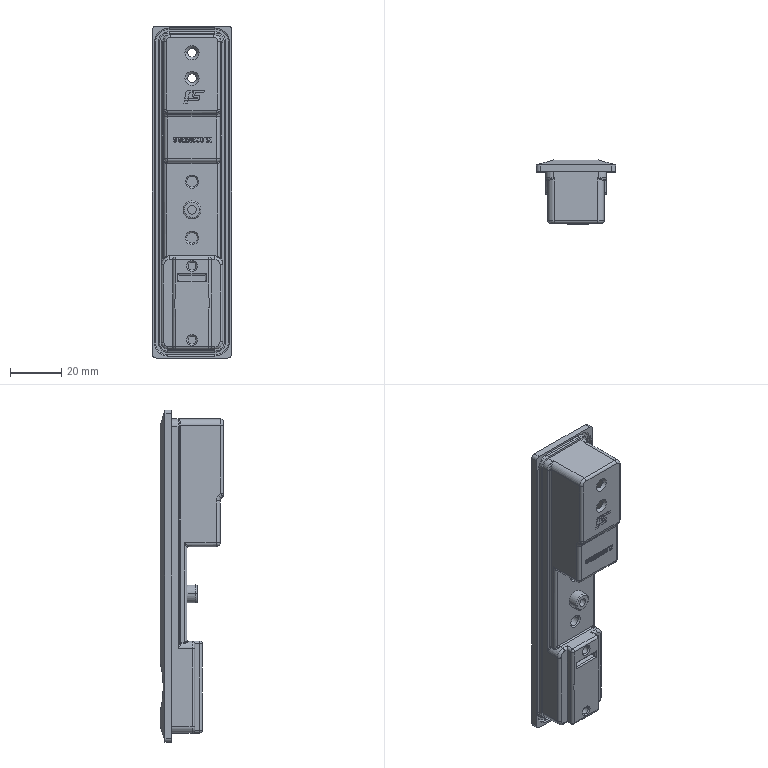Part | STEP file | _X2_751F4E45_X0_MS731-1_X2_8_13 | 1 solid | 721 faces | box 31 x 25.045 x 130 mm | volume 21766 mm3 | plane 491 | cylinder 145 | torus 39 | sphere 18 | spline 16 | cone 12 | commonest cylinder face diameters 1 x55 2 x23 3 x13 6 x5 2.8 x4 3.2 x4